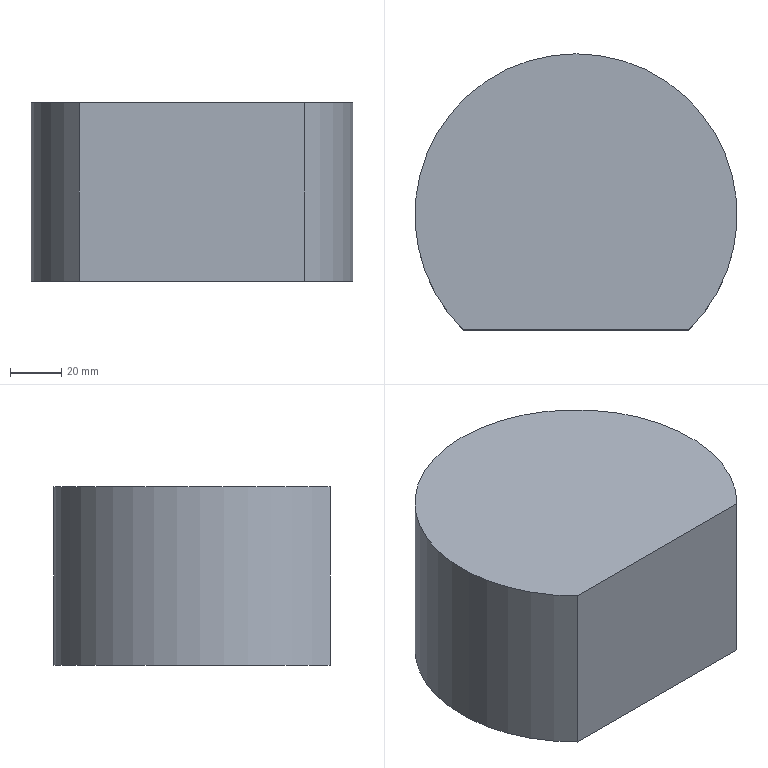Part | NX | features solid 2 | 1 solid | 6 faces | box 126 x 108 x 70 mm | volume 713248 mm3 | plane 4 | cylinder 2 | commonest cylinder face diameters 46 x1 126 x1
STEP:
#1=CARTESIAN_POINT('',(-415.909,-335.,75.));
#2=VERTEX_POINT('',#1);
#3=CARTESIAN_POINT('',(-415.909,-335.,145.));
#4=VERTEX_POINT('',#3);
#5=CARTESIAN_POINT('',(-415.909,-335.,75.));
#6=DIRECTION('',(0.,0.,1.));
#7=VECTOR('',#6,1000.);
#8=LINE('',#5,#7);
#9=EDGE_CURVE('',#2,#4,#8,.T.);
#10=ORIENTED_EDGE('',*,*,#9,.F.);
#11=CARTESIAN_POINT('',(-504.091,-335.,75.));
#12=VERTEX_POINT('',#11);
#13=CARTESIAN_POINT('',(-460.,-290.,75.));
#14=DIRECTION('',(0.,0.,-1.));
#15=DIRECTION('',(-1.,0.,0.));
#16=AXIS2_PLACEMENT_3D('',#13,#14,#15);
#17=CIRCLE('',#16,63.);
#18=EDGE_CURVE('',#12,#2,#17,.T.);
#19=ORIENTED_EDGE('',*,*,#18,.F.);
#20=CARTESIAN_POINT('',(-504.091,-335.,145.));
#21=VERTEX_POINT('',#20);
#22=CARTESIAN_POINT('',(-504.091,-335.,75.));
#23=DIRECTION('',(0.,0.,1.));
#24=VECTOR('',#23,1000.);
#25=LINE('',#22,#24);
#26=EDGE_CURVE('',#21,#12,#25,.F.);
#27=ORIENTED_EDGE('',*,*,#26,.F.);
#28=CARTESIAN_POINT('',(-460.,-290.,145.));
#29=DIRECTION('',(0.,0.,-1.));
#30=DIRECTION('',(-1.,0.,0.));
#31=AXIS2_PLACEMENT_3D('',#28,#29,#30);
#32=CIRCLE('',#31,63.);
#33=EDGE_CURVE('',#21,#4,#32,.T.);
#34=ORIENTED_EDGE('',*,*,#33,.T.);
#35=EDGE_LOOP('',(#10,#19,#27,#34));
#36=FACE_BOUND('',#35,.T.);
#37=CARTESIAN_POINT('',(-460.,-290.,75.));
#38=DIRECTION('',(0.,0.,1.));
#39=DIRECTION('',(1.,0.,0.));
#40=AXIS2_PLACEMENT_3D('',#37,#38,#39);
#41=CYLINDRICAL_SURFACE('',#40,63.);
#42=ADVANCED_FACE('',(#36),#41,.T.);
#43=CARTESIAN_POINT('',(-483.,-290.,75.));
#44=VERTEX_POINT('',#43);
#45=CARTESIAN_POINT('',(-460.,-290.,75.));
#46=DIRECTION('',(0.,0.,-1.));
#47=DIRECTION('',(-1.,0.,0.));
#48=AXIS2_PLACEMENT_3D('',#45,#46,#47);
#49=CIRCLE('',#48,23.);
#50=EDGE_CURVE('',#44,#44,#49,.T.);
#51=ORIENTED_EDGE('',*,*,#50,.F.);
#52=EDGE_LOOP('',(#51));
#53=FACE_BOUND('',#52,.T.);
#54=ORIENTED_EDGE('',*,*,#18,.T.);
#55=CARTESIAN_POINT('',(-460.,-335.,75.));
#56=DIRECTION('',(-1.,0.,0.));
#57=VECTOR('',#56,1000.);
#58=LINE('',#55,#57);
#59=EDGE_CURVE('',#2,#12,#58,.T.);
#60=ORIENTED_EDGE('',*,*,#59,.T.);
#61=EDGE_LOOP('',(#54,#60));
#62=FACE_BOUND('',#61,.T.);
#63=CARTESIAN_POINT('',(-460.,-290.,75.));
#64=DIRECTION('',(0.,0.,-1.));
#65=DIRECTION('',(-1.,0.,0.));
#66=AXIS2_PLACEMENT_3D('',#63,#64,#65);
#67=PLANE('',#66);
#68=ADVANCED_FACE('',(#53,#62),#67,.T.);
#69=CARTESIAN_POINT('',(-460.,-335.,145.));
#70=DIRECTION('',(-1.,0.,0.));
#71=VECTOR('',#70,1000.);
#72=LINE('',#69,#71);
#73=EDGE_CURVE('',#4,#21,#72,.T.);
#74=ORIENTED_EDGE('',*,*,#73,.F.);
#75=ORIENTED_EDGE('',*,*,#33,.F.);
#76=EDGE_LOOP('',(#74,#75));
#77=FACE_BOUND('',#76,.T.);
#78=CARTESIAN_POINT('',(-460.,-290.,145.));
#79=DIRECTION('',(0.,0.,-1.));
#80=DIRECTION('',(-1.,0.,0.));
#81=AXIS2_PLACEMENT_3D('',#78,#79,#80);
#82=PLANE('',#81);
#83=ADVANCED_FACE('',(#77),#82,.F.);
#84=ORIENTED_EDGE('',*,*,#50,.T.);
#85=EDGE_LOOP('',(#84));
#86=FACE_BOUND('',#85,.T.);
#87=CARTESIAN_POINT('',(-483.,-290.,125.));
#88=VERTEX_POINT('',#87);
#89=CARTESIAN_POINT('',(-460.,-290.,125.));
#90=DIRECTION('',(0.,0.,-1.));
#91=DIRECTION('',(-1.,0.,0.));
#92=AXIS2_PLACEMENT_3D('',#89,#90,#91);
#93=CIRCLE('',#92,23.);
#94=EDGE_CURVE('',#88,#88,#93,.T.);
#95=ORIENTED_EDGE('',*,*,#94,.F.);
#96=EDGE_LOOP('',(#95));
#97=FACE_BOUND('',#96,.T.);
#98=CARTESIAN_POINT('',(-460.,-290.,75.));
#99=DIRECTION('',(0.,0.,1.));
#100=DIRECTION('',(1.,0.,0.));
#101=AXIS2_PLACEMENT_3D('',#98,#99,#100);
#102=CYLINDRICAL_SURFACE('',#101,23.);
#103=ADVANCED_FACE('',(#86,#97),#102,.F.);
#104=ORIENTED_EDGE('',*,*,#94,.T.);
#105=EDGE_LOOP('',(#104));
#106=FACE_BOUND('',#105,.T.);
#107=CARTESIAN_POINT('',(-460.,-290.,125.));
#108=DIRECTION('',(0.,0.,-1.));
#109=DIRECTION('',(-1.,0.,0.));
#110=AXIS2_PLACEMENT_3D('',#107,#108,#109);
#111=PLANE('',#110);
#112=ADVANCED_FACE('',(#106),#111,.T.);
#113=ORIENTED_EDGE('',*,*,#59,.F.);
#114=ORIENTED_EDGE('',*,*,#9,.T.);
#115=ORIENTED_EDGE('',*,*,#73,.T.);
#116=ORIENTED_EDGE('',*,*,#26,.T.);
#117=EDGE_LOOP('',(#113,#114,#115,#116));
#118=FACE_BOUND('',#117,.T.);
#119=CARTESIAN_POINT('',(-495.,-335.,340.));
#120=DIRECTION('',(0.,-1.,0.));
#121=DIRECTION('',(0.,0.,-1.));
#122=AXIS2_PLACEMENT_3D('',#119,#120,#121);
#123=PLANE('',#122);
#124=ADVANCED_FACE('',(#118),#123,.T.);
#125=CLOSED_SHELL('',(#42,#68,#83,#103,#112,#124));
#126=MANIFOLD_SOLID_BREP('',#125);
#127=(LENGTH_UNIT()NAMED_UNIT(*)SI_UNIT(.MILLI.,.METRE.));
#128=UNCERTAINTY_MEASURE_WITH_UNIT(LENGTH_MEASURE(0.00001),#127,'','');
#129=(NAMED_UNIT(*)PLANE_ANGLE_UNIT()SI_UNIT($,.RADIAN.));
#130=(NAMED_UNIT(*)SI_UNIT($,.STERADIAN.)SOLID_ANGLE_UNIT());
#131=(GEOMETRIC_REPRESENTATION_CONTEXT(3)GLOBAL_UNCERTAINTY_ASSIGNED_CONTEXT((#128))GLOBAL_UNIT_ASSIGNED_CONTEXT((#127,#129,#130))REPRESENTATION_CONTEXT('',''));
#132=ADVANCED_BREP_SHAPE_REPRESENTATION('',(#126),#131);